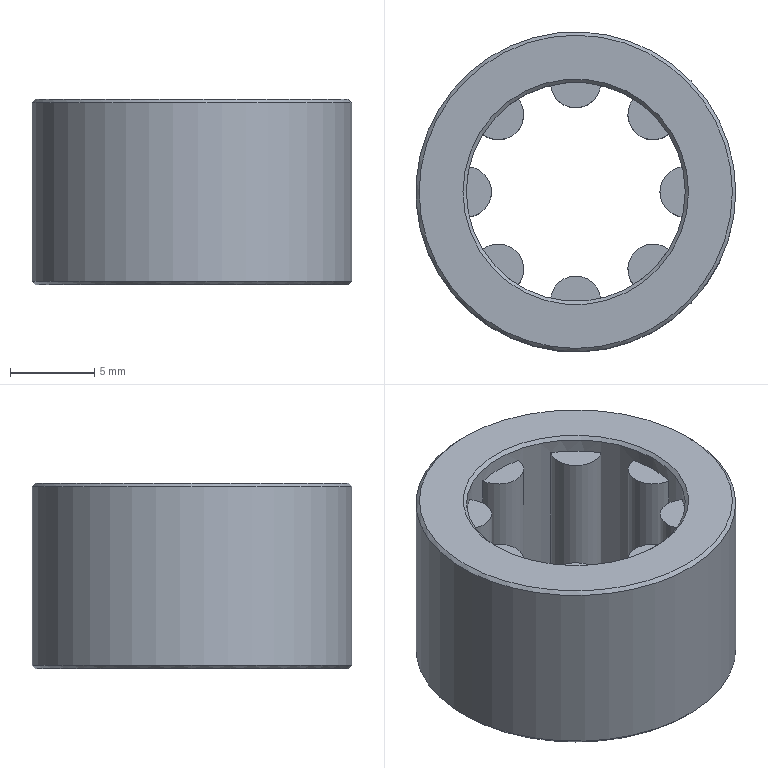Part | NX | features BREP 1 | 1 solid | 32 faces | box 19 x 19 x 11 mm | volume 1897 mm3 | plane 18 | cylinder 10 | cone 4 | commonest cylinder face diameters 3 x8 13 x1 19 x1
STEP:
#1=CARTESIAN_POINT('',(6.7,0.,11.));
#2=VERTEX_POINT('',#1);
#3=CARTESIAN_POINT('',(0.,0.,11.));
#4=DIRECTION('',(0.,0.,-1.));
#5=DIRECTION('',(1.,0.,0.));
#6=AXIS2_PLACEMENT_3D('',#3,#4,#5);
#7=CIRCLE('',#6,6.7);
#8=EDGE_CURVE('',#2,#2,#7,.T.);
#9=ORIENTED_EDGE('',*,*,#8,.F.);
#10=EDGE_LOOP('',(#9));
#11=FACE_BOUND('',#10,.T.);
#12=CARTESIAN_POINT('',(6.5,0.,10.8));
#13=VERTEX_POINT('',#12);
#14=CARTESIAN_POINT('',(0.,0.,10.8));
#15=DIRECTION('',(0.,0.,1.));
#16=DIRECTION('',(1.,0.,0.));
#17=AXIS2_PLACEMENT_3D('',#14,#15,#16);
#18=CIRCLE('',#17,6.5);
#19=EDGE_CURVE('',#13,#13,#18,.T.);
#20=ORIENTED_EDGE('',*,*,#19,.F.);
#21=EDGE_LOOP('',(#20));
#22=FACE_BOUND('',#21,.T.);
#23=CARTESIAN_POINT('',(0.,0.,11.));
#24=DIRECTION('',(0.,0.,1.));
#25=DIRECTION('',(1.,0.,0.));
#26=AXIS2_PLACEMENT_3D('',#23,#24,#25);
#27=CONICAL_SURFACE('',#26,6.7,0.7854);
#28=ADVANCED_FACE('',(#11,#22),#27,.F.);
#29=CARTESIAN_POINT('',(6.7,0.,0.));
#30=VERTEX_POINT('',#29);
#31=CARTESIAN_POINT('',(0.,0.,0.));
#32=DIRECTION('',(0.,0.,1.));
#33=DIRECTION('',(1.,0.,0.));
#34=AXIS2_PLACEMENT_3D('',#31,#32,#33);
#35=CIRCLE('',#34,6.7);
#36=EDGE_CURVE('',#30,#30,#35,.T.);
#37=ORIENTED_EDGE('',*,*,#36,.F.);
#38=EDGE_LOOP('',(#37));
#39=FACE_BOUND('',#38,.T.);
#40=CARTESIAN_POINT('',(6.5,0.,0.2));
#41=VERTEX_POINT('',#40);
#42=CARTESIAN_POINT('',(0.,0.,0.2));
#43=DIRECTION('',(0.,0.,-1.));
#44=DIRECTION('',(1.,0.,0.));
#45=AXIS2_PLACEMENT_3D('',#42,#43,#44);
#46=CIRCLE('',#45,6.5);
#47=EDGE_CURVE('',#41,#41,#46,.T.);
#48=ORIENTED_EDGE('',*,*,#47,.F.);
#49=EDGE_LOOP('',(#48));
#50=FACE_BOUND('',#49,.T.);
#51=CARTESIAN_POINT('',(0.,0.,0.2));
#52=DIRECTION('',(0.,0.,-1.));
#53=DIRECTION('',(-1.,0.,0.));
#54=AXIS2_PLACEMENT_3D('',#51,#52,#53);
#55=CONICAL_SURFACE('',#54,6.5,0.7854);
#56=ADVANCED_FACE('',(#39,#50),#55,.F.);
#57=CARTESIAN_POINT('',(9.5,0.,10.8));
#58=VERTEX_POINT('',#57);
#59=CARTESIAN_POINT('',(0.,0.,10.8));
#60=DIRECTION('',(0.,0.,-1.));
#61=DIRECTION('',(1.,0.,0.));
#62=AXIS2_PLACEMENT_3D('',#59,#60,#61);
#63=CIRCLE('',#62,9.5);
#64=EDGE_CURVE('',#58,#58,#63,.T.);
#65=ORIENTED_EDGE('',*,*,#64,.F.);
#66=EDGE_LOOP('',(#65));
#67=FACE_BOUND('',#66,.T.);
#68=CARTESIAN_POINT('',(9.3,0.,11.));
#69=VERTEX_POINT('',#68);
#70=CARTESIAN_POINT('',(0.,0.,11.));
#71=DIRECTION('',(0.,0.,1.));
#72=DIRECTION('',(1.,0.,0.));
#73=AXIS2_PLACEMENT_3D('',#70,#71,#72);
#74=CIRCLE('',#73,9.3);
#75=EDGE_CURVE('',#69,#69,#74,.T.);
#76=ORIENTED_EDGE('',*,*,#75,.F.);
#77=EDGE_LOOP('',(#76));
#78=FACE_BOUND('',#77,.T.);
#79=CARTESIAN_POINT('',(0.,0.,11.));
#80=DIRECTION('',(0.,0.,-1.));
#81=DIRECTION('',(-1.,0.,0.));
#82=AXIS2_PLACEMENT_3D('',#79,#80,#81);
#83=CONICAL_SURFACE('',#82,9.3,0.7854);
#84=ADVANCED_FACE('',(#67,#78),#83,.T.);
#85=CARTESIAN_POINT('',(9.5,0.,0.2));
#86=VERTEX_POINT('',#85);
#87=CARTESIAN_POINT('',(0.,0.,0.2));
#88=DIRECTION('',(0.,0.,1.));
#89=DIRECTION('',(1.,0.,0.));
#90=AXIS2_PLACEMENT_3D('',#87,#88,#89);
#91=CIRCLE('',#90,9.5);
#92=EDGE_CURVE('',#86,#86,#91,.T.);
#93=ORIENTED_EDGE('',*,*,#92,.F.);
#94=EDGE_LOOP('',(#93));
#95=FACE_BOUND('',#94,.T.);
#96=CARTESIAN_POINT('',(9.3,0.,0.));
#97=VERTEX_POINT('',#96);
#98=CARTESIAN_POINT('',(0.,0.,0.));
#99=DIRECTION('',(0.,0.,-1.));
#100=DIRECTION('',(1.,0.,0.));
#101=AXIS2_PLACEMENT_3D('',#98,#99,#100);
#102=CIRCLE('',#101,9.3);
#103=EDGE_CURVE('',#97,#97,#102,.T.);
#104=ORIENTED_EDGE('',*,*,#103,.F.);
#105=EDGE_LOOP('',(#104));
#106=FACE_BOUND('',#105,.T.);
#107=CARTESIAN_POINT('',(0.,0.,0.2));
#108=DIRECTION('',(0.,0.,1.));
#109=DIRECTION('',(1.,0.,0.));
#110=AXIS2_PLACEMENT_3D('',#107,#108,#109);
#111=CONICAL_SURFACE('',#110,9.5,0.7854);
#112=ADVANCED_FACE('',(#95,#106),#111,.T.);
#113=ORIENTED_EDGE('',*,*,#47,.T.);
#114=EDGE_LOOP('',(#113));
#115=FACE_BOUND('',#114,.T.);
#116=CARTESIAN_POINT('',(-6.327,1.49,10.));
#117=VERTEX_POINT('',#116);
#118=CARTESIAN_POINT('',(-6.327,-1.49,10.));
#119=VERTEX_POINT('',#118);
#120=CARTESIAN_POINT('',(0.,0.,10.));
#121=DIRECTION('',(0.,0.,1.));
#122=DIRECTION('',(1.,0.,0.));
#123=AXIS2_PLACEMENT_3D('',#120,#121,#122);
#124=CIRCLE('',#123,6.5);
#125=EDGE_CURVE('',#117,#119,#124,.T.);
#126=ORIENTED_EDGE('',*,*,#125,.F.);
#127=CARTESIAN_POINT('',(-6.327,1.49,1.));
#128=VERTEX_POINT('',#127);
#129=CARTESIAN_POINT('',(-6.327,1.49,11.));
#130=DIRECTION('',(0.,0.,-1.));
#131=VECTOR('',#130,1000.);
#132=LINE('',#129,#131);
#133=EDGE_CURVE('',#128,#117,#132,.F.);
#134=ORIENTED_EDGE('',*,*,#133,.F.);
#135=CARTESIAN_POINT('',(-6.327,-1.49,1.));
#136=VERTEX_POINT('',#135);
#137=CARTESIAN_POINT('',(0.,0.,1.));
#138=DIRECTION('',(0.,0.,-1.));
#139=DIRECTION('',(-1.,0.,0.));
#140=AXIS2_PLACEMENT_3D('',#137,#138,#139);
#141=CIRCLE('',#140,6.5);
#142=EDGE_CURVE('',#136,#128,#141,.T.);
#143=ORIENTED_EDGE('',*,*,#142,.F.);
#144=CARTESIAN_POINT('',(-6.327,-1.49,11.));
#145=DIRECTION('',(0.,0.,-1.));
#146=VECTOR('',#145,1000.);
#147=LINE('',#144,#146);
#148=EDGE_CURVE('',#136,#119,#147,.F.);
#149=ORIENTED_EDGE('',*,*,#148,.T.);
#150=EDGE_LOOP('',(#126,#134,#143,#149));
#151=FACE_BOUND('',#150,.T.);
#152=ORIENTED_EDGE('',*,*,#19,.T.);
#153=EDGE_LOOP('',(#152));
#154=FACE_BOUND('',#153,.T.);
#155=CARTESIAN_POINT('',(5.527,-3.42,1.));
#156=VERTEX_POINT('',#155);
#157=CARTESIAN_POINT('',(3.42,-5.527,1.));
#158=VERTEX_POINT('',#157);
#159=CARTESIAN_POINT('',(0.,0.,1.));
#160=DIRECTION('',(0.,0.,-1.));
#161=DIRECTION('',(-1.,0.,0.));
#162=AXIS2_PLACEMENT_3D('',#159,#160,#161);
#163=CIRCLE('',#162,6.5);
#164=EDGE_CURVE('',#156,#158,#163,.T.);
#165=ORIENTED_EDGE('',*,*,#164,.F.);
#166=CARTESIAN_POINT('',(5.527,-3.42,10.));
#167=VERTEX_POINT('',#166);
#168=CARTESIAN_POINT('',(5.527,-3.42,11.));
#169=DIRECTION('',(0.,0.,-1.));
#170=VECTOR('',#169,1000.);
#171=LINE('',#168,#170);
#172=EDGE_CURVE('',#167,#156,#171,.T.);
#173=ORIENTED_EDGE('',*,*,#172,.F.);
#174=CARTESIAN_POINT('',(3.42,-5.527,10.));
#175=VERTEX_POINT('',#174);
#176=CARTESIAN_POINT('',(0.,0.,10.));
#177=DIRECTION('',(0.,0.,1.));
#178=DIRECTION('',(1.,0.,0.));
#179=AXIS2_PLACEMENT_3D('',#176,#177,#178);
#180=CIRCLE('',#179,6.5);
#181=EDGE_CURVE('',#175,#167,#180,.T.);
#182=ORIENTED_EDGE('',*,*,#181,.F.);
#183=CARTESIAN_POINT('',(3.42,-5.527,11.));
#184=DIRECTION('',(0.,0.,-1.));
#185=VECTOR('',#184,1000.);
#186=LINE('',#183,#185);
#187=EDGE_CURVE('',#175,#158,#186,.T.);
#188=ORIENTED_EDGE('',*,*,#187,.T.);
#189=EDGE_LOOP('',(#165,#173,#182,#188));
#190=FACE_BOUND('',#189,.T.);
#191=CARTESIAN_POINT('',(1.49,-6.327,1.));
#192=VERTEX_POINT('',#191);
#193=CARTESIAN_POINT('',(-1.49,-6.327,1.));
#194=VERTEX_POINT('',#193);
#195=CARTESIAN_POINT('',(0.,0.,1.));
#196=DIRECTION('',(0.,0.,-1.));
#197=DIRECTION('',(-1.,0.,0.));
#198=AXIS2_PLACEMENT_3D('',#195,#196,#197);
#199=CIRCLE('',#198,6.5);
#200=EDGE_CURVE('',#192,#194,#199,.T.);
#201=ORIENTED_EDGE('',*,*,#200,.F.);
#202=CARTESIAN_POINT('',(1.49,-6.327,10.));
#203=VERTEX_POINT('',#202);
#204=CARTESIAN_POINT('',(1.49,-6.327,11.));
#205=DIRECTION('',(0.,0.,-1.));
#206=VECTOR('',#205,1000.);
#207=LINE('',#204,#206);
#208=EDGE_CURVE('',#203,#192,#207,.T.);
#209=ORIENTED_EDGE('',*,*,#208,.F.);
#210=CARTESIAN_POINT('',(-1.49,-6.327,10.));
#211=VERTEX_POINT('',#210);
#212=CARTESIAN_POINT('',(0.,0.,10.));
#213=DIRECTION('',(0.,0.,1.));
#214=DIRECTION('',(1.,0.,0.));
#215=AXIS2_PLACEMENT_3D('',#212,#213,#214);
#216=CIRCLE('',#215,6.5);
#217=EDGE_CURVE('',#211,#203,#216,.T.);
#218=ORIENTED_EDGE('',*,*,#217,.F.);
#219=CARTESIAN_POINT('',(-1.49,-6.327,11.));
#220=DIRECTION('',(0.,0.,-1.));
#221=VECTOR('',#220,1000.);
#222=LINE('',#219,#221);
#223=EDGE_CURVE('',#211,#194,#222,.T.);
#224=ORIENTED_EDGE('',*,*,#223,.T.);
#225=EDGE_LOOP('',(#201,#209,#218,#224));
#226=FACE_BOUND('',#225,.T.);
#227=CARTESIAN_POINT('',(-3.42,-5.527,1.));
#228=VERTEX_POINT('',#227);
#229=CARTESIAN_POINT('',(-5.527,-3.42,1.));
#230=VERTEX_POINT('',#229);
#231=CARTESIAN_POINT('',(0.,0.,1.));
#232=DIRECTION('',(0.,0.,-1.));
#233=DIRECTION('',(-1.,0.,0.));
#234=AXIS2_PLACEMENT_3D('',#231,#232,#233);
#235=CIRCLE('',#234,6.5);
#236=EDGE_CURVE('',#228,#230,#235,.T.);
#237=ORIENTED_EDGE('',*,*,#236,.F.);
#238=CARTESIAN_POINT('',(-3.42,-5.527,10.));
#239=VERTEX_POINT('',#238);
#240=CARTESIAN_POINT('',(-3.42,-5.527,11.));
#241=DIRECTION('',(0.,0.,-1.));
#242=VECTOR('',#241,1000.);
#243=LINE('',#240,#242);
#244=EDGE_CURVE('',#239,#228,#243,.T.);
#245=ORIENTED_EDGE('',*,*,#244,.F.);
#246=CARTESIAN_POINT('',(-5.527,-3.42,10.));
#247=VERTEX_POINT('',#246);
#248=CARTESIAN_POINT('',(0.,0.,10.));
#249=DIRECTION('',(0.,0.,1.));
#250=DIRECTION('',(1.,0.,0.));
#251=AXIS2_PLACEMENT_3D('',#248,#249,#250);
#252=CIRCLE('',#251,6.5);
#253=EDGE_CURVE('',#247,#239,#252,.T.);
#254=ORIENTED_EDGE('',*,*,#253,.F.);
#255=CARTESIAN_POINT('',(-5.527,-3.42,11.));
#256=DIRECTION('',(0.,0.,-1.));
#257=VECTOR('',#256,1000.);
#258=LINE('',#255,#257);
#259=EDGE_CURVE('',#247,#230,#258,.T.);
#260=ORIENTED_EDGE('',*,*,#259,.T.);
#261=EDGE_LOOP('',(#237,#245,#254,#260));
#262=FACE_BOUND('',#261,.T.);
#263=CARTESIAN_POINT('',(6.327,1.49,1.));
#264=VERTEX_POINT('',#263);
#265=CARTESIAN_POINT('',(6.327,-1.49,1.));
#266=VERTEX_POINT('',#265);
#267=CARTESIAN_POINT('',(0.,0.,1.));
#268=DIRECTION('',(0.,0.,-1.));
#269=DIRECTION('',(-1.,0.,0.));
#270=AXIS2_PLACEMENT_3D('',#267,#268,#269);
#271=CIRCLE('',#270,6.5);
#272=EDGE_CURVE('',#264,#266,#271,.T.);
#273=ORIENTED_EDGE('',*,*,#272,.F.);
#274=CARTESIAN_POINT('',(6.327,1.49,10.));
#275=VERTEX_POINT('',#274);
#276=CARTESIAN_POINT('',(6.327,1.49,11.));
#277=DIRECTION('',(0.,0.,-1.));
#278=VECTOR('',#277,1000.);
#279=LINE('',#276,#278);
#280=EDGE_CURVE('',#275,#264,#279,.T.);
#281=ORIENTED_EDGE('',*,*,#280,.F.);
#282=CARTESIAN_POINT('',(6.327,-1.49,10.));
#283=VERTEX_POINT('',#282);
#284=CARTESIAN_POINT('',(0.,0.,10.));
#285=DIRECTION('',(0.,0.,1.));
#286=DIRECTION('',(1.,0.,0.));
#287=AXIS2_PLACEMENT_3D('',#284,#285,#286);
#288=CIRCLE('',#287,6.5);
#289=EDGE_CURVE('',#283,#275,#288,.T.);
#290=ORIENTED_EDGE('',*,*,#289,.F.);
#291=CARTESIAN_POINT('',(6.327,-1.49,11.));
#292=DIRECTION('',(0.,0.,-1.));
#293=VECTOR('',#292,1000.);
#294=LINE('',#291,#293);
#295=EDGE_CURVE('',#283,#266,#294,.T.);
#296=ORIENTED_EDGE('',*,*,#295,.T.);
#297=EDGE_LOOP('',(#273,#281,#290,#296));
#298=FACE_BOUND('',#297,.T.);
#299=CARTESIAN_POINT('',(-5.527,3.42,1.));
#300=VERTEX_POINT('',#299);
#301=CARTESIAN_POINT('',(-3.42,5.527,1.));
#302=VERTEX_POINT('',#301);
#303=CARTESIAN_POINT('',(0.,0.,1.));
#304=DIRECTION('',(0.,0.,-1.));
#305=DIRECTION('',(-1.,0.,0.));
#306=AXIS2_PLACEMENT_3D('',#303,#304,#305);
#307=CIRCLE('',#306,6.5);
#308=EDGE_CURVE('',#300,#302,#307,.T.);
#309=ORIENTED_EDGE('',*,*,#308,.F.);
#310=CARTESIAN_POINT('',(-5.527,3.42,10.));
#311=VERTEX_POINT('',#310);
#312=CARTESIAN_POINT('',(-5.527,3.42,11.));
#313=DIRECTION('',(0.,0.,-1.));
#314=VECTOR('',#313,1000.);
#315=LINE('',#312,#314);
#316=EDGE_CURVE('',#300,#311,#315,.F.);
#317=ORIENTED_EDGE('',*,*,#316,.T.);
#318=CARTESIAN_POINT('',(-3.42,5.527,10.));
#319=VERTEX_POINT('',#318);
#320=CARTESIAN_POINT('',(0.,0.,10.));
#321=DIRECTION('',(0.,0.,1.));
#322=DIRECTION('',(1.,0.,0.));
#323=AXIS2_PLACEMENT_3D('',#320,#321,#322);
#324=CIRCLE('',#323,6.5);
#325=EDGE_CURVE('',#319,#311,#324,.T.);
#326=ORIENTED_EDGE('',*,*,#325,.F.);
#327=CARTESIAN_POINT('',(-3.42,5.527,11.));
#328=DIRECTION('',(0.,0.,-1.));
#329=VECTOR('',#328,1000.);
#330=LINE('',#327,#329);
#331=EDGE_CURVE('',#302,#319,#330,.F.);
#332=ORIENTED_EDGE('',*,*,#331,.F.);
#333=EDGE_LOOP('',(#309,#317,#326,#332));
#334=FACE_BOUND('',#333,.T.);
#335=CARTESIAN_POINT('',(3.42,5.527,1.));
#336=VERTEX_POINT('',#335);
#337=CARTESIAN_POINT('',(5.527,3.42,1.));
#338=VERTEX_POINT('',#337);
#339=CARTESIAN_POINT('',(0.,0.,1.));
#340=DIRECTION('',(0.,0.,-1.));
#341=DIRECTION('',(-1.,0.,0.));
#342=AXIS2_PLACEMENT_3D('',#339,#340,#341);
#343=CIRCLE('',#342,6.5);
#344=EDGE_CURVE('',#336,#338,#343,.T.);
#345=ORIENTED_EDGE('',*,*,#344,.F.);
#346=CARTESIAN_POINT('',(3.42,5.527,10.));
#347=VERTEX_POINT('',#346);
#348=CARTESIAN_POINT('',(3.42,5.527,11.));
#349=DIRECTION('',(0.,0.,-1.));
#350=VECTOR('',#349,1000.);
#351=LINE('',#348,#350);
#352=EDGE_CURVE('',#336,#347,#351,.F.);
#353=ORIENTED_EDGE('',*,*,#352,.T.);
#354=CARTESIAN_POINT('',(5.527,3.42,10.));
#355=VERTEX_POINT('',#354);
#356=CARTESIAN_POINT('',(0.,0.,10.));
#357=DIRECTION('',(0.,0.,1.));
#358=DIRECTION('',(1.,0.,0.));
#359=AXIS2_PLACEMENT_3D('',#356,#357,#358);
#360=CIRCLE('',#359,6.5);
#361=EDGE_CURVE('',#355,#347,#360,.T.);
#362=ORIENTED_EDGE('',*,*,#361,.F.);
#363=CARTESIAN_POINT('',(5.527,3.42,11.));
#364=DIRECTION('',(0.,0.,-1.));
#365=VECTOR('',#364,1000.);
#366=LINE('',#363,#365);
#367=EDGE_CURVE('',#338,#355,#366,.F.);
#368=ORIENTED_EDGE('',*,*,#367,.F.);
#369=EDGE_LOOP('',(#345,#353,#362,#368));
#370=FACE_BOUND('',#369,.T.);
#371=CARTESIAN_POINT('',(-1.49,6.327,1.));
#372=VERTEX_POINT('',#371);
#373=CARTESIAN_POINT('',(1.49,6.327,1.));
#374=VERTEX_POINT('',#373);
#375=CARTESIAN_POINT('',(0.,0.,1.));
#376=DIRECTION('',(0.,0.,-1.));
#377=DIRECTION('',(-1.,0.,0.));
#378=AXIS2_PLACEMENT_3D('',#375,#376,#377);
#379=CIRCLE('',#378,6.5);
#380=EDGE_CURVE('',#372,#374,#379,.T.);
#381=ORIENTED_EDGE('',*,*,#380,.F.);
#382=CARTESIAN_POINT('',(-1.49,6.327,10.));
#383=VERTEX_POINT('',#382);
#384=CARTESIAN_POINT('',(-1.49,6.327,11.));
#385=DIRECTION('',(0.,0.,-1.));
#386=VECTOR('',#385,1000.);
#387=LINE('',#384,#386);
#388=EDGE_CURVE('',#372,#383,#387,.F.);
#389=ORIENTED_EDGE('',*,*,#388,.T.);
#390=CARTESIAN_POINT('',(1.49,6.327,10.));
#391=VERTEX_POINT('',#390);
#392=CARTESIAN_POINT('',(0.,0.,10.));
#393=DIRECTION('',(0.,0.,1.));
#394=DIRECTION('',(1.,0.,0.));
#395=AXIS2_PLACEMENT_3D('',#392,#393,#394);
#396=CIRCLE('',#395,6.5);
#397=EDGE_CURVE('',#391,#383,#396,.T.);
#398=ORIENTED_EDGE('',*,*,#397,.F.);
#399=CARTESIAN_POINT('',(1.49,6.327,11.));
#400=DIRECTION('',(0.,0.,-1.));
#401=VECTOR('',#400,1000.);
#402=LINE('',#399,#401);
#403=EDGE_CURVE('',#374,#391,#402,.F.);
#404=ORIENTED_EDGE('',*,*,#403,.F.);
#405=EDGE_LOOP('',(#381,#389,#398,#404));
#406=FACE_BOUND('',#405,.T.);
#407=CARTESIAN_POINT('',(0.,0.,11.));
#408=DIRECTION('',(0.,0.,-1.));
#409=DIRECTION('',(-1.,0.,0.));
#410=AXIS2_PLACEMENT_3D('',#407,#408,#409);
#411=CYLINDRICAL_SURFACE('',#410,6.5);
#412=ADVANCED_FACE('',(#115,#151,#154,#190,#226,#262,#298,#334,#370,#406),#411,.F.);
#413=ORIENTED_EDGE('',*,*,#92,.T.);
#414=EDGE_LOOP('',(#413));
#415=FACE_BOUND('',#414,.T.);
#416=ORIENTED_EDGE('',*,*,#64,.T.);
#417=EDGE_LOOP('',(#416));
#418=FACE_BOUND('',#417,.T.);
#419=CARTESIAN_POINT('',(0.,0.,11.));
#420=DIRECTION('',(0.,0.,-1.));
#421=DIRECTION('',(-1.,0.,0.));
#422=AXIS2_PLACEMENT_3D('',#419,#420,#421);
#423=CYLINDRICAL_SURFACE('',#422,9.5);
#424=ADVANCED_FACE('',(#415,#418),#423,.T.);
#425=CARTESIAN_POINT('',(4.596,4.596,10.));
#426=DIRECTION('',(0.,0.,1.));
#427=DIRECTION('',(1.,0.,0.));
#428=AXIS2_PLACEMENT_3D('',#425,#426,#427);
#429=CIRCLE('',#428,1.5);
#430=EDGE_CURVE('',#347,#355,#429,.T.);
#431=ORIENTED_EDGE('',*,*,#430,.F.);
#432=ORIENTED_EDGE('',*,*,#352,.F.);
#433=CARTESIAN_POINT('',(4.596,4.596,1.));
#434=DIRECTION('',(0.,0.,-1.));
#435=DIRECTION('',(-1.,0.,0.));
#436=AXIS2_PLACEMENT_3D('',#433,#434,#435);
#437=CIRCLE('',#436,1.5);
#438=EDGE_CURVE('',#338,#336,#437,.T.);
#439=ORIENTED_EDGE('',*,*,#438,.F.);
#440=ORIENTED_EDGE('',*,*,#367,.T.);
#441=EDGE_LOOP('',(#431,#432,#439,#440));
#442=FACE_BOUND('',#441,.T.);
#443=CARTESIAN_POINT('',(4.596,4.596,11.));
#444=DIRECTION('',(0.,0.,-1.));
#445=DIRECTION('',(-1.,0.,0.));
#446=AXIS2_PLACEMENT_3D('',#443,#444,#445);
#447=CYLINDRICAL_SURFACE('',#446,1.5);
#448=ADVANCED_FACE('',(#442),#447,.T.);
#449=CARTESIAN_POINT('',(6.5,0.,10.));
#450=DIRECTION('',(0.,0.,1.));
#451=DIRECTION('',(1.,0.,0.));
#452=AXIS2_PLACEMENT_3D('',#449,#450,#451);
#453=CIRCLE('',#452,1.5);
#454=EDGE_CURVE('',#275,#283,#453,.T.);
#455=ORIENTED_EDGE('',*,*,#454,.F.);
#456=ORIENTED_EDGE('',*,*,#280,.T.);
#457=CARTESIAN_POINT('',(6.5,0.,1.));
#458=DIRECTION('',(0.,0.,-1.));
#459=DIRECTION('',(-1.,0.,0.));
#460=AXIS2_PLACEMENT_3D('',#457,#458,#459);
#461=CIRCLE('',#460,1.5);
#462=EDGE_CURVE('',#266,#264,#461,.T.);
#463=ORIENTED_EDGE('',*,*,#462,.F.);
#464=ORIENTED_EDGE('',*,*,#295,.F.);
#465=EDGE_LOOP('',(#455,#456,#463,#464));
#466=FACE_BOUND('',#465,.T.);
#467=CARTESIAN_POINT('',(6.5,0.,11.));
#468=DIRECTION('',(0.,0.,-1.));
#469=DIRECTION('',(-1.,0.,0.));
#470=AXIS2_PLACEMENT_3D('',#467,#468,#469);
#471=CYLINDRICAL_SURFACE('',#470,1.5);
#472=ADVANCED_FACE('',(#466),#471,.T.);
#473=CARTESIAN_POINT('',(4.596,-4.596,10.));
#474=DIRECTION('',(0.,0.,1.));
#475=DIRECTION('',(1.,0.,0.));
#476=AXIS2_PLACEMENT_3D('',#473,#474,#475);
#477=CIRCLE('',#476,1.5);
#478=EDGE_CURVE('',#167,#175,#477,.T.);
#479=ORIENTED_EDGE('',*,*,#478,.F.);
#480=ORIENTED_EDGE('',*,*,#172,.T.);
#481=CARTESIAN_POINT('',(4.596,-4.596,1.));
#482=DIRECTION('',(0.,0.,-1.));
#483=DIRECTION('',(-1.,0.,0.));
#484=AXIS2_PLACEMENT_3D('',#481,#482,#483);
#485=CIRCLE('',#484,1.5);
#486=EDGE_CURVE('',#158,#156,#485,.T.);
#487=ORIENTED_EDGE('',*,*,#486,.F.);
#488=ORIENTED_EDGE('',*,*,#187,.F.);
#489=EDGE_LOOP('',(#479,#480,#487,#488));
#490=FACE_BOUND('',#489,.T.);
#491=CARTESIAN_POINT('',(4.596,-4.596,11.));
#492=DIRECTION('',(0.,0.,-1.));
#493=DIRECTION('',(-1.,0.,0.));
#494=AXIS2_PLACEMENT_3D('',#491,#492,#493);
#495=CYLINDRICAL_SURFACE('',#494,1.5);
#496=ADVANCED_FACE('',(#490),#495,.T.);
#497=CARTESIAN_POINT('',(-4.596,4.596,1.));
#498=DIRECTION('',(0.,0.,-1.));
#499=DIRECTION('',(-1.,0.,0.));
#500=AXIS2_PLACEMENT_3D('',#497,#498,#499);
#501=CIRCLE('',#500,1.5);
#502=EDGE_CURVE('',#302,#300,#501,.T.);
#503=ORIENTED_EDGE('',*,*,#502,.F.);
#504=ORIENTED_EDGE('',*,*,#331,.T.);
#505=CARTESIAN_POINT('',(-4.596,4.596,10.));
#506=DIRECTION('',(0.,0.,1.));
#507=DIRECTION('',(1.,0.,0.));
#508=AXIS2_PLACEMENT_3D('',#505,#506,#507);
#509=CIRCLE('',#508,1.5);
#510=EDGE_CURVE('',#311,#319,#509,.T.);
#511=ORIENTED_EDGE('',*,*,#510,.F.);
#512=ORIENTED_EDGE('',*,*,#316,.F.);
#513=EDGE_LOOP('',(#503,#504,#511,#512));
#514=FACE_BOUND('',#513,.T.);
#515=CARTESIAN_POINT('',(-4.596,4.596,11.));
#516=DIRECTION('',(0.,0.,-1.));
#517=DIRECTION('',(-1.,0.,0.));
#518=AXIS2_PLACEMENT_3D('',#515,#516,#517);
#519=CYLINDRICAL_SURFACE('',#518,1.5);
#520=ADVANCED_FACE('',(#514),#519,.T.);
#521=CARTESIAN_POINT('',(-6.5,0.,1.));
#522=DIRECTION('',(0.,0.,-1.));
#523=DIRECTION('',(-1.,0.,0.));
#524=AXIS2_PLACEMENT_3D('',#521,#522,#523);
#525=CIRCLE('',#524,1.5);
#526=EDGE_CURVE('',#128,#136,#525,.T.);
#527=ORIENTED_EDGE('',*,*,#526,.F.);
#528=ORIENTED_EDGE('',*,*,#133,.T.);
#529=CARTESIAN_POINT('',(-6.5,0.,10.));
#530=DIRECTION('',(0.,0.,1.));
#531=DIRECTION('',(1.,0.,0.));
#532=AXIS2_PLACEMENT_3D('',#529,#530,#531);
#533=CIRCLE('',#532,1.5);
#534=EDGE_CURVE('',#119,#117,#533,.T.);
#535=ORIENTED_EDGE('',*,*,#534,.F.);
#536=ORIENTED_EDGE('',*,*,#148,.F.);
#537=EDGE_LOOP('',(#527,#528,#535,#536));
#538=FACE_BOUND('',#537,.T.);
#539=CARTESIAN_POINT('',(-6.5,0.,11.));
#540=DIRECTION('',(0.,0.,-1.));
#541=DIRECTION('',(-1.,0.,0.));
#542=AXIS2_PLACEMENT_3D('',#539,#540,#541);
#543=CYLINDRICAL_SURFACE('',#542,1.5);
#544=ADVANCED_FACE('',(#538),#543,.T.);
#545=CARTESIAN_POINT('',(-4.596,-4.596,1.));
#546=DIRECTION('',(0.,0.,-1.));
#547=DIRECTION('',(-1.,0.,0.));
#548=AXIS2_PLACEMENT_3D('',#545,#546,#547);
#549=CIRCLE('',#548,1.5);
#550=EDGE_CURVE('',#230,#228,#549,.T.);
#551=ORIENTED_EDGE('',*,*,#550,.F.);
#552=ORIENTED_EDGE('',*,*,#259,.F.);
#553=CARTESIAN_POINT('',(-4.596,-4.596,10.));
#554=DIRECTION('',(0.,0.,1.));
#555=DIRECTION('',(1.,0.,0.));
#556=AXIS2_PLACEMENT_3D('',#553,#554,#555);
#557=CIRCLE('',#556,1.5);
#558=EDGE_CURVE('',#239,#247,#557,.T.);
#559=ORIENTED_EDGE('',*,*,#558,.F.);
#560=ORIENTED_EDGE('',*,*,#244,.T.);
#561=EDGE_LOOP('',(#551,#552,#559,#560));
#562=FACE_BOUND('',#561,.T.);
#563=CARTESIAN_POINT('',(-4.596,-4.596,11.));
#564=DIRECTION('',(0.,0.,-1.));
#565=DIRECTION('',(-1.,0.,0.));
#566=AXIS2_PLACEMENT_3D('',#563,#564,#565);
#567=CYLINDRICAL_SURFACE('',#566,1.5);
#568=ADVANCED_FACE('',(#562),#567,.T.);
#569=CARTESIAN_POINT('',(0.,-6.5,1.));
#570=DIRECTION('',(0.,0.,-1.));
#571=DIRECTION('',(-1.,0.,0.));
#572=AXIS2_PLACEMENT_3D('',#569,#570,#571);
#573=CIRCLE('',#572,1.5);
#574=EDGE_CURVE('',#194,#192,#573,.T.);
#575=ORIENTED_EDGE('',*,*,#574,.F.);
#576=ORIENTED_EDGE('',*,*,#223,.F.);
#577=CARTESIAN_POINT('',(0.,-6.5,10.));
#578=DIRECTION('',(0.,0.,1.));
#579=DIRECTION('',(1.,0.,0.));
#580=AXIS2_PLACEMENT_3D('',#577,#578,#579);
#581=CIRCLE('',#580,1.5);
#582=EDGE_CURVE('',#203,#211,#581,.T.);
#583=ORIENTED_EDGE('',*,*,#582,.F.);
#584=ORIENTED_EDGE('',*,*,#208,.T.);
#585=EDGE_LOOP('',(#575,#576,#583,#584));
#586=FACE_BOUND('',#585,.T.);
#587=CARTESIAN_POINT('',(0.,-6.5,11.));
#588=DIRECTION('',(0.,0.,-1.));
#589=DIRECTION('',(-1.,0.,0.));
#590=AXIS2_PLACEMENT_3D('',#587,#588,#589);
#591=CYLINDRICAL_SURFACE('',#590,1.5);
#592=ADVANCED_FACE('',(#586),#591,.T.);
#593=CARTESIAN_POINT('',(0.,6.5,1.));
#594=DIRECTION('',(0.,0.,-1.));
#595=DIRECTION('',(-1.,0.,0.));
#596=AXIS2_PLACEMENT_3D('',#593,#594,#595);
#597=CIRCLE('',#596,1.5);
#598=EDGE_CURVE('',#374,#372,#597,.T.);
#599=ORIENTED_EDGE('',*,*,#598,.F.);
#600=ORIENTED_EDGE('',*,*,#403,.T.);
#601=CARTESIAN_POINT('',(0.,6.5,10.));
#602=DIRECTION('',(0.,0.,1.));
#603=DIRECTION('',(1.,0.,0.));
#604=AXIS2_PLACEMENT_3D('',#601,#602,#603);
#605=CIRCLE('',#604,1.5);
#606=EDGE_CURVE('',#383,#391,#605,.T.);
#607=ORIENTED_EDGE('',*,*,#606,.F.);
#608=ORIENTED_EDGE('',*,*,#388,.F.);
#609=EDGE_LOOP('',(#599,#600,#607,#608));
#610=FACE_BOUND('',#609,.T.);
#611=CARTESIAN_POINT('',(0.,6.5,11.));
#612=DIRECTION('',(0.,0.,-1.));
#613=DIRECTION('',(-1.,0.,0.));
#614=AXIS2_PLACEMENT_3D('',#611,#612,#613);
#615=CYLINDRICAL_SURFACE('',#614,1.5);
#616=ADVANCED_FACE('',(#610),#615,.T.);
#617=ORIENTED_EDGE('',*,*,#75,.T.);
#618=EDGE_LOOP('',(#617));
#619=FACE_BOUND('',#618,.T.);
#620=ORIENTED_EDGE('',*,*,#8,.T.);
#621=EDGE_LOOP('',(#620));
#622=FACE_BOUND('',#621,.T.);
#623=CARTESIAN_POINT('',(0.,0.,11.));
#624=DIRECTION('',(0.,0.,1.));
#625=DIRECTION('',(1.,0.,0.));
#626=AXIS2_PLACEMENT_3D('',#623,#624,#625);
#627=PLANE('',#626);
#628=ADVANCED_FACE('',(#619,#622),#627,.T.);
#629=ORIENTED_EDGE('',*,*,#103,.T.);
#630=EDGE_LOOP('',(#629));
#631=FACE_BOUND('',#630,.T.);
#632=ORIENTED_EDGE('',*,*,#36,.T.);
#633=EDGE_LOOP('',(#632));
#634=FACE_BOUND('',#633,.T.);
#635=CARTESIAN_POINT('',(0.,0.,0.));
#636=DIRECTION('',(0.,0.,1.));
#637=DIRECTION('',(1.,0.,0.));
#638=AXIS2_PLACEMENT_3D('',#635,#636,#637);
#639=PLANE('',#638);
#640=ADVANCED_FACE('',(#631,#634),#639,.F.);
#641=ORIENTED_EDGE('',*,*,#606,.T.);
#642=ORIENTED_EDGE('',*,*,#397,.T.);
#643=EDGE_LOOP('',(#641,#642));
#644=FACE_BOUND('',#643,.T.);
#645=CARTESIAN_POINT('',(0.,0.,10.));
#646=DIRECTION('',(0.,0.,1.));
#647=DIRECTION('',(1.,0.,0.));
#648=AXIS2_PLACEMENT_3D('',#645,#646,#647);
#649=PLANE('',#648);
#650=ADVANCED_FACE('',(#644),#649,.T.);
#651=ORIENTED_EDGE('',*,*,#361,.T.);
#652=ORIENTED_EDGE('',*,*,#430,.T.);
#653=EDGE_LOOP('',(#651,#652));
#654=FACE_BOUND('',#653,.T.);
#655=CARTESIAN_POINT('',(0.,0.,10.));
#656=DIRECTION('',(0.,0.,1.));
#657=DIRECTION('',(1.,0.,0.));
#658=AXIS2_PLACEMENT_3D('',#655,#656,#657);
#659=PLANE('',#658);
#660=ADVANCED_FACE('',(#654),#659,.T.);
#661=ORIENTED_EDGE('',*,*,#289,.T.);
#662=ORIENTED_EDGE('',*,*,#454,.T.);
#663=EDGE_LOOP('',(#661,#662));
#664=FACE_BOUND('',#663,.T.);
#665=CARTESIAN_POINT('',(0.,0.,10.));
#666=DIRECTION('',(0.,0.,1.));
#667=DIRECTION('',(1.,0.,0.));
#668=AXIS2_PLACEMENT_3D('',#665,#666,#667);
#669=PLANE('',#668);
#670=ADVANCED_FACE('',(#664),#669,.T.);
#671=ORIENTED_EDGE('',*,*,#181,.T.);
#672=ORIENTED_EDGE('',*,*,#478,.T.);
#673=EDGE_LOOP('',(#671,#672));
#674=FACE_BOUND('',#673,.T.);
#675=CARTESIAN_POINT('',(0.,0.,10.));
#676=DIRECTION('',(0.,0.,1.));
#677=DIRECTION('',(1.,0.,0.));
#678=AXIS2_PLACEMENT_3D('',#675,#676,#677);
#679=PLANE('',#678);
#680=ADVANCED_FACE('',(#674),#679,.T.);
#681=ORIENTED_EDGE('',*,*,#582,.T.);
#682=ORIENTED_EDGE('',*,*,#217,.T.);
#683=EDGE_LOOP('',(#681,#682));
#684=FACE_BOUND('',#683,.T.);
#685=CARTESIAN_POINT('',(0.,0.,10.));
#686=DIRECTION('',(0.,0.,1.));
#687=DIRECTION('',(1.,0.,0.));
#688=AXIS2_PLACEMENT_3D('',#685,#686,#687);
#689=PLANE('',#688);
#690=ADVANCED_FACE('',(#684),#689,.T.);
#691=ORIENTED_EDGE('',*,*,#558,.T.);
#692=ORIENTED_EDGE('',*,*,#253,.T.);
#693=EDGE_LOOP('',(#691,#692));
#694=FACE_BOUND('',#693,.T.);
#695=CARTESIAN_POINT('',(0.,0.,10.));
#696=DIRECTION('',(0.,0.,1.));
#697=DIRECTION('',(1.,0.,0.));
#698=AXIS2_PLACEMENT_3D('',#695,#696,#697);
#699=PLANE('',#698);
#700=ADVANCED_FACE('',(#694),#699,.T.);
#701=ORIENTED_EDGE('',*,*,#534,.T.);
#702=ORIENTED_EDGE('',*,*,#125,.T.);
#703=EDGE_LOOP('',(#701,#702));
#704=FACE_BOUND('',#703,.T.);
#705=CARTESIAN_POINT('',(0.,0.,10.));
#706=DIRECTION('',(0.,0.,1.));
#707=DIRECTION('',(1.,0.,0.));
#708=AXIS2_PLACEMENT_3D('',#705,#706,#707);
#709=PLANE('',#708);
#710=ADVANCED_FACE('',(#704),#709,.T.);
#711=ORIENTED_EDGE('',*,*,#510,.T.);
#712=ORIENTED_EDGE('',*,*,#325,.T.);
#713=EDGE_LOOP('',(#711,#712));
#714=FACE_BOUND('',#713,.T.);
#715=CARTESIAN_POINT('',(0.,0.,10.));
#716=DIRECTION('',(0.,0.,1.));
#717=DIRECTION('',(1.,0.,0.));
#718=AXIS2_PLACEMENT_3D('',#715,#716,#717);
#719=PLANE('',#718);
#720=ADVANCED_FACE('',(#714),#719,.T.);
#721=ORIENTED_EDGE('',*,*,#462,.T.);
#722=ORIENTED_EDGE('',*,*,#272,.T.);
#723=EDGE_LOOP('',(#721,#722));
#724=FACE_BOUND('',#723,.T.);
#725=CARTESIAN_POINT('',(0.,0.,1.));
#726=DIRECTION('',(0.,0.,-1.));
#727=DIRECTION('',(-1.,0.,0.));
#728=AXIS2_PLACEMENT_3D('',#725,#726,#727);
#729=PLANE('',#728);
#730=ADVANCED_FACE('',(#724),#729,.T.);
#731=ORIENTED_EDGE('',*,*,#486,.T.);
#732=ORIENTED_EDGE('',*,*,#164,.T.);
#733=EDGE_LOOP('',(#731,#732));
#734=FACE_BOUND('',#733,.T.);
#735=CARTESIAN_POINT('',(0.,0.,1.));
#736=DIRECTION('',(0.,0.,-1.));
#737=DIRECTION('',(-1.,0.,0.));
#738=AXIS2_PLACEMENT_3D('',#735,#736,#737);
#739=PLANE('',#738);
#740=ADVANCED_FACE('',(#734),#739,.T.);
#741=ORIENTED_EDGE('',*,*,#574,.T.);
#742=ORIENTED_EDGE('',*,*,#200,.T.);
#743=EDGE_LOOP('',(#741,#742));
#744=FACE_BOUND('',#743,.T.);
#745=CARTESIAN_POINT('',(0.,0.,1.));
#746=DIRECTION('',(0.,0.,-1.));
#747=DIRECTION('',(-1.,0.,0.));
#748=AXIS2_PLACEMENT_3D('',#745,#746,#747);
#749=PLANE('',#748);
#750=ADVANCED_FACE('',(#744),#749,.T.);
#751=ORIENTED_EDGE('',*,*,#550,.T.);
#752=ORIENTED_EDGE('',*,*,#236,.T.);
#753=EDGE_LOOP('',(#751,#752));
#754=FACE_BOUND('',#753,.T.);
#755=CARTESIAN_POINT('',(0.,0.,1.));
#756=DIRECTION('',(0.,0.,-1.));
#757=DIRECTION('',(-1.,0.,0.));
#758=AXIS2_PLACEMENT_3D('',#755,#756,#757);
#759=PLANE('',#758);
#760=ADVANCED_FACE('',(#754),#759,.T.);
#761=ORIENTED_EDGE('',*,*,#526,.T.);
#762=ORIENTED_EDGE('',*,*,#142,.T.);
#763=EDGE_LOOP('',(#761,#762));
#764=FACE_BOUND('',#763,.T.);
#765=CARTESIAN_POINT('',(0.,0.,1.));
#766=DIRECTION('',(0.,0.,-1.));
#767=DIRECTION('',(-1.,0.,0.));
#768=AXIS2_PLACEMENT_3D('',#765,#766,#767);
#769=PLANE('',#768);
#770=ADVANCED_FACE('',(#764),#769,.T.);
#771=ORIENTED_EDGE('',*,*,#502,.T.);
#772=ORIENTED_EDGE('',*,*,#308,.T.);
#773=EDGE_LOOP('',(#771,#772));
#774=FACE_BOUND('',#773,.T.);
#775=CARTESIAN_POINT('',(0.,0.,1.));
#776=DIRECTION('',(0.,0.,-1.));
#777=DIRECTION('',(-1.,0.,0.));
#778=AXIS2_PLACEMENT_3D('',#775,#776,#777);
#779=PLANE('',#778);
#780=ADVANCED_FACE('',(#774),#779,.T.);
#781=ORIENTED_EDGE('',*,*,#598,.T.);
#782=ORIENTED_EDGE('',*,*,#380,.T.);
#783=EDGE_LOOP('',(#781,#782));
#784=FACE_BOUND('',#783,.T.);
#785=CARTESIAN_POINT('',(0.,0.,1.));
#786=DIRECTION('',(0.,0.,-1.));
#787=DIRECTION('',(-1.,0.,0.));
#788=AXIS2_PLACEMENT_3D('',#785,#786,#787);
#789=PLANE('',#788);
#790=ADVANCED_FACE('',(#784),#789,.T.);
#791=ORIENTED_EDGE('',*,*,#438,.T.);
#792=ORIENTED_EDGE('',*,*,#344,.T.);
#793=EDGE_LOOP('',(#791,#792));
#794=FACE_BOUND('',#793,.T.);
#795=CARTESIAN_POINT('',(0.,0.,1.));
#796=DIRECTION('',(0.,0.,-1.));
#797=DIRECTION('',(-1.,0.,0.));
#798=AXIS2_PLACEMENT_3D('',#795,#796,#797);
#799=PLANE('',#798);
#800=ADVANCED_FACE('',(#794),#799,.T.);
#801=CLOSED_SHELL('',(#28,#56,#84,#112,#412,#424,#448,#472,#496,#520,#544,#568,#592,#616,#628,#640,#650,#660,#670,#680,#690,#700,#710,#720,#730,#740,#750,#760,#770,#780,#790,#800));
#802=MANIFOLD_SOLID_BREP('',#801);
#803=(LENGTH_UNIT()NAMED_UNIT(*)SI_UNIT(.MILLI.,.METRE.));
#804=UNCERTAINTY_MEASURE_WITH_UNIT(LENGTH_MEASURE(0.00001),#803,'','');
#805=(NAMED_UNIT(*)PLANE_ANGLE_UNIT()SI_UNIT($,.RADIAN.));
#806=(NAMED_UNIT(*)SI_UNIT($,.STERADIAN.)SOLID_ANGLE_UNIT());
#807=(GEOMETRIC_REPRESENTATION_CONTEXT(3)GLOBAL_UNCERTAINTY_ASSIGNED_CONTEXT((#804))GLOBAL_UNIT_ASSIGNED_CONTEXT((#803,#805,#806))REPRESENTATION_CONTEXT('',''));
#808=ADVANCED_BREP_SHAPE_REPRESENTATION('',(#802),#807);